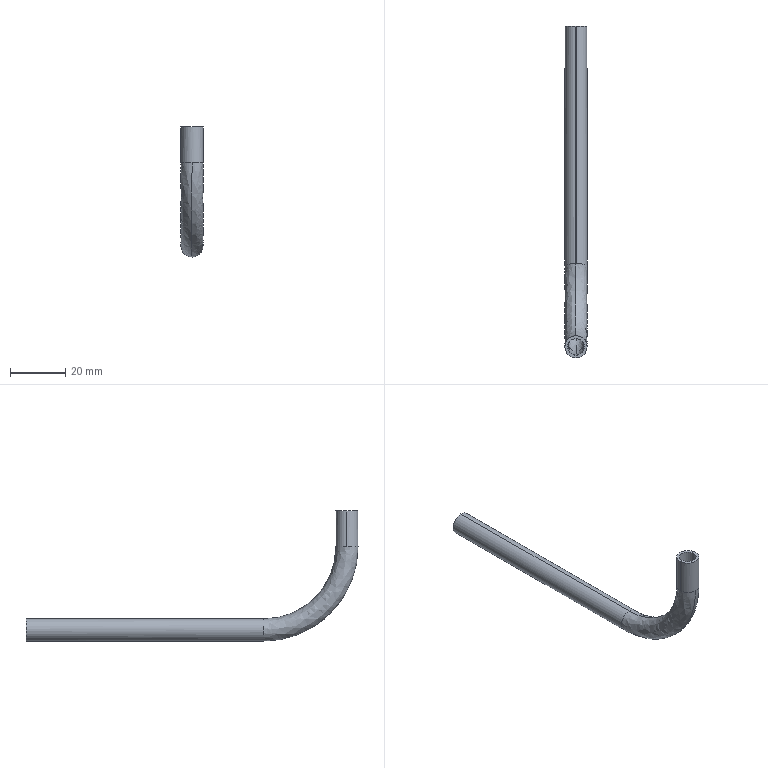Part | SolidWorks | features BaseBody 1 | 1 solid | 14 faces | box 8 x 120 x 47 mm | volume 3213 mm3 | cylinder 8 | spline 4 | plane 2 | commonest cylinder face diameters 6 x4 8 x4
STEP:
#1=CARTESIAN_POINT('',(-48.,-40.,-43.));
#2=VERTEX_POINT('',#1);
#3=CARTESIAN_POINT('',(-44.,-40.,-39.));
#4=VERTEX_POINT('',#3);
#5=CARTESIAN_POINT('',(-48.,-40.,-39.));
#6=DIRECTION('',(0.,-1.,0.));
#7=DIRECTION('',(0.,0.,-1.));
#8=AXIS2_PLACEMENT_3D('',#5,#6,#7);
#9=CIRCLE('',#8,4.);
#10=EDGE_CURVE('',#2,#4,#9,.T.);
#11=ORIENTED_EDGE('',*,*,#10,.F.);
#12=CARTESIAN_POINT('',(-48.,46.,-43.));
#13=VERTEX_POINT('',#12);
#14=CARTESIAN_POINT('',(-48.,-40.,-43.));
#15=DIRECTION('',(0.,1.,0.));
#16=VECTOR('',#15,1000.);
#17=LINE('',#14,#16);
#18=EDGE_CURVE('',#2,#13,#17,.T.);
#19=ORIENTED_EDGE('',*,*,#18,.T.);
#20=CARTESIAN_POINT('',(-48.,46.,-35.));
#21=VERTEX_POINT('',#20);
#22=CARTESIAN_POINT('',(-48.,46.,-39.));
#23=DIRECTION('',(0.,-1.,0.));
#24=DIRECTION('',(0.,0.,1.));
#25=AXIS2_PLACEMENT_3D('',#22,#23,#24);
#26=CIRCLE('',#25,4.);
#27=EDGE_CURVE('',#13,#21,#26,.T.);
#28=ORIENTED_EDGE('',*,*,#27,.T.);
#29=CARTESIAN_POINT('',(-48.,-40.,-35.));
#30=VERTEX_POINT('',#29);
#31=CARTESIAN_POINT('',(-48.,-40.,-35.));
#32=DIRECTION('',(0.,1.,0.));
#33=VECTOR('',#32,1000.);
#34=LINE('',#31,#33);
#35=EDGE_CURVE('',#30,#21,#34,.T.);
#36=ORIENTED_EDGE('',*,*,#35,.F.);
#37=CARTESIAN_POINT('',(-48.,-40.,-39.));
#38=DIRECTION('',(0.,1.,0.));
#39=DIRECTION('',(0.,0.,1.));
#40=AXIS2_PLACEMENT_3D('',#37,#38,#39);
#41=CIRCLE('',#40,4.);
#42=EDGE_CURVE('',#30,#4,#41,.T.);
#43=ORIENTED_EDGE('',*,*,#42,.T.);
#44=EDGE_LOOP('',(#11,#19,#28,#36,#43));
#45=FACE_OUTER_BOUND('',#44,.T.);
#46=CARTESIAN_POINT('',(-48.,-40.,-39.));
#47=DIRECTION('',(0.,1.,0.));
#48=DIRECTION('',(0.,0.,1.));
#49=AXIS2_PLACEMENT_3D('',#46,#47,#48);
#50=CYLINDRICAL_SURFACE('',#49,4.);
#51=ADVANCED_FACE('',(#45),#50,.T.);
#52=CARTESIAN_POINT('',(-52.,-70.,-9.));
#53=VERTEX_POINT('',#52);
#54=CARTESIAN_POINT('',(-48.001,-66.,-9.));
#55=VERTEX_POINT('',#54);
#56=CARTESIAN_POINT('',(-48.,-70.,-9.));
#57=DIRECTION('',(0.,0.,-1.));
#58=DIRECTION('',(0.,-1.,0.));
#59=AXIS2_PLACEMENT_3D('',#56,#57,#58);
#60=CIRCLE('',#59,4.);
#61=EDGE_CURVE('',#53,#55,#60,.T.);
#62=ORIENTED_EDGE('',*,*,#61,.F.);
#63=CARTESIAN_POINT('',(-52.,-70.,4.));
#64=VERTEX_POINT('',#63);
#65=CARTESIAN_POINT('',(-52.,-70.,-9.));
#66=DIRECTION('',(0.,0.,1.));
#67=VECTOR('',#66,1000.);
#68=LINE('',#65,#67);
#69=EDGE_CURVE('',#53,#64,#68,.T.);
#70=ORIENTED_EDGE('',*,*,#69,.T.);
#71=CARTESIAN_POINT('',(-44.,-70.,4.));
#72=VERTEX_POINT('',#71);
#73=CARTESIAN_POINT('',(-48.,-70.,4.));
#74=DIRECTION('',(0.,0.,-1.));
#75=DIRECTION('',(1.,0.,0.));
#76=AXIS2_PLACEMENT_3D('',#73,#74,#75);
#77=CIRCLE('',#76,4.);
#78=EDGE_CURVE('',#64,#72,#77,.T.);
#79=ORIENTED_EDGE('',*,*,#78,.T.);
#80=CARTESIAN_POINT('',(-44.,-70.,-9.));
#81=VERTEX_POINT('',#80);
#82=CARTESIAN_POINT('',(-44.,-70.,-9.));
#83=DIRECTION('',(0.,0.,1.));
#84=VECTOR('',#83,1000.);
#85=LINE('',#82,#84);
#86=EDGE_CURVE('',#81,#72,#85,.T.);
#87=ORIENTED_EDGE('',*,*,#86,.F.);
#88=CARTESIAN_POINT('',(-48.,-70.,-9.));
#89=DIRECTION('',(0.,0.,-1.));
#90=DIRECTION('',(0.,-1.,0.));
#91=AXIS2_PLACEMENT_3D('',#88,#89,#90);
#92=CIRCLE('',#91,4.);
#93=EDGE_CURVE('',#55,#81,#92,.T.);
#94=ORIENTED_EDGE('',*,*,#93,.F.);
#95=EDGE_LOOP('',(#62,#70,#79,#87,#94));
#96=FACE_OUTER_BOUND('',#95,.T.);
#97=CARTESIAN_POINT('',(-48.,-70.,-9.));
#98=DIRECTION('',(0.,0.,1.));
#99=DIRECTION('',(1.,0.,0.));
#100=AXIS2_PLACEMENT_3D('',#97,#98,#99);
#101=CYLINDRICAL_SURFACE('',#100,4.);
#102=ADVANCED_FACE('',(#96),#101,.T.);
#103=CARTESIAN_POINT('',(-48.,-40.,-42.));
#104=VERTEX_POINT('',#103);
#105=CARTESIAN_POINT('',(-48.,-40.,-36.));
#106=VERTEX_POINT('',#105);
#107=CARTESIAN_POINT('',(-48.,-40.,-39.));
#108=DIRECTION('',(0.,1.,0.));
#109=DIRECTION('',(0.,0.,1.));
#110=AXIS2_PLACEMENT_3D('',#107,#108,#109);
#111=CIRCLE('',#110,3.);
#112=EDGE_CURVE('',#104,#106,#111,.T.);
#113=ORIENTED_EDGE('',*,*,#112,.F.);
#114=CARTESIAN_POINT('',(-48.,46.,-42.));
#115=VERTEX_POINT('',#114);
#116=CARTESIAN_POINT('',(-48.,-40.,-42.));
#117=DIRECTION('',(0.,1.,0.));
#118=VECTOR('',#117,1000.);
#119=LINE('',#116,#118);
#120=EDGE_CURVE('',#104,#115,#119,.T.);
#121=ORIENTED_EDGE('',*,*,#120,.T.);
#122=CARTESIAN_POINT('',(-48.,46.,-36.));
#123=VERTEX_POINT('',#122);
#124=CARTESIAN_POINT('',(-48.,46.,-39.));
#125=DIRECTION('',(0.,-1.,0.));
#126=DIRECTION('',(0.,0.,1.));
#127=AXIS2_PLACEMENT_3D('',#124,#125,#126);
#128=CIRCLE('',#127,3.);
#129=EDGE_CURVE('',#123,#115,#128,.T.);
#130=ORIENTED_EDGE('',*,*,#129,.F.);
#131=CARTESIAN_POINT('',(-48.,-40.,-36.));
#132=DIRECTION('',(0.,1.,0.));
#133=VECTOR('',#132,1000.);
#134=LINE('',#131,#133);
#135=EDGE_CURVE('',#106,#123,#134,.T.);
#136=ORIENTED_EDGE('',*,*,#135,.F.);
#137=EDGE_LOOP('',(#113,#121,#130,#136));
#138=FACE_OUTER_BOUND('',#137,.T.);
#139=CARTESIAN_POINT('',(-48.,-40.,-39.));
#140=DIRECTION('',(0.,1.,0.));
#141=DIRECTION('',(0.,0.,1.));
#142=AXIS2_PLACEMENT_3D('',#139,#140,#141);
#143=CYLINDRICAL_SURFACE('',#142,3.);
#144=ADVANCED_FACE('',(#138),#143,.F.);
#145=CARTESIAN_POINT('',(-48.,-67.,-9.));
#146=VERTEX_POINT('',#145);
#147=CARTESIAN_POINT('',(-45.,-70.,-9.));
#148=VERTEX_POINT('',#147);
#149=CARTESIAN_POINT('',(-48.,-70.,-9.));
#150=DIRECTION('',(0.,0.,-1.));
#151=DIRECTION('',(0.,-1.,0.));
#152=AXIS2_PLACEMENT_3D('',#149,#150,#151);
#153=CIRCLE('',#152,3.);
#154=EDGE_CURVE('',#146,#148,#153,.T.);
#155=ORIENTED_EDGE('',*,*,#154,.F.);
#156=CARTESIAN_POINT('',(-48.,-40.,-9.));
#157=DIRECTION('',(1.,0.,0.));
#158=DIRECTION('',(0.,-1.,0.));
#159=AXIS2_PLACEMENT_3D('',#156,#157,#158);
#160=CIRCLE('',#159,27.);
#161=EDGE_CURVE('',#146,#106,#160,.T.);
#162=ORIENTED_EDGE('',*,*,#161,.T.);
#163=CARTESIAN_POINT('',(-48.,-40.,-39.));
#164=DIRECTION('',(0.,1.,0.));
#165=DIRECTION('',(0.,0.,1.));
#166=AXIS2_PLACEMENT_3D('',#163,#164,#165);
#167=CIRCLE('',#166,3.);
#168=EDGE_CURVE('',#106,#104,#167,.T.);
#169=ORIENTED_EDGE('',*,*,#168,.T.);
#170=CARTESIAN_POINT('',(-48.,-73.,-9.));
#171=VERTEX_POINT('',#170);
#172=CARTESIAN_POINT('',(-48.,-40.,-9.));
#173=DIRECTION('',(1.,0.,0.));
#174=DIRECTION('',(0.,-1.,0.));
#175=AXIS2_PLACEMENT_3D('',#172,#173,#174);
#176=CIRCLE('',#175,33.);
#177=EDGE_CURVE('',#171,#104,#176,.T.);
#178=ORIENTED_EDGE('',*,*,#177,.F.);
#179=CARTESIAN_POINT('',(-48.,-70.,-9.));
#180=DIRECTION('',(0.,0.,-1.));
#181=DIRECTION('',(0.,-1.,0.));
#182=AXIS2_PLACEMENT_3D('',#179,#180,#181);
#183=CIRCLE('',#182,3.);
#184=EDGE_CURVE('',#148,#171,#183,.T.);
#185=ORIENTED_EDGE('',*,*,#184,.F.);
#186=EDGE_LOOP('',(#155,#162,#169,#178,#185));
#187=FACE_OUTER_BOUND('',#186,.T.);
#188=CARTESIAN_POINT('',(-48.,-67.,-9.));
#189=CARTESIAN_POINT('',(-48.,-67.,-24.816));
#190=CARTESIAN_POINT('',(-48.,-55.816,-36.));
#191=CARTESIAN_POINT('',(-48.,-40.,-36.));
#192=CARTESIAN_POINT('',(-42.,-67.,-9.));
#193=CARTESIAN_POINT('',(-42.,-67.,-24.816));
#194=CARTESIAN_POINT('',(-42.,-55.816,-36.));
#195=CARTESIAN_POINT('',(-42.,-40.,-36.));
#196=CARTESIAN_POINT('',(-42.,-73.,-9.));
#197=CARTESIAN_POINT('',(-42.,-73.,-28.331));
#198=CARTESIAN_POINT('',(-42.,-59.331,-42.));
#199=CARTESIAN_POINT('',(-42.,-40.,-42.));
#200=CARTESIAN_POINT('',(-48.,-73.,-9.));
#201=CARTESIAN_POINT('',(-48.,-73.,-28.331));
#202=CARTESIAN_POINT('',(-48.,-59.331,-42.));
#203=CARTESIAN_POINT('',(-48.,-40.,-42.));
#204=(BOUNDED_SURFACE()B_SPLINE_SURFACE(3,3,((#188,#189,#190,#191),(#192,#193,#194,#195),(#196,#197,#198,#199),(#200,#201,#202,#203)),.UNSPECIFIED.,.F.,.F.,.T.)B_SPLINE_SURFACE_WITH_KNOTS((4,4),(4,4),(0.,1.),(0.,1.),.UNSPECIFIED.)GEOMETRIC_REPRESENTATION_ITEM()RATIONAL_B_SPLINE_SURFACE(((1.,0.8047,0.8047,1.),(0.3333,0.2682,0.2682,0.3333),(0.3333,0.2682,0.2682,0.3333),(1.,0.8047,0.8047,1.)))REPRESENTATION_ITEM('')SURFACE());
#205=ADVANCED_FACE('',(#187),#204,.F.);
#206=ORIENTED_EDGE('',*,*,#184,.T.);
#207=CARTESIAN_POINT('',(-51.,-70.,-9.));
#208=VERTEX_POINT('',#207);
#209=CARTESIAN_POINT('',(-48.,-70.,-9.));
#210=DIRECTION('',(0.,0.,-1.));
#211=DIRECTION('',(0.,-1.,0.));
#212=AXIS2_PLACEMENT_3D('',#209,#210,#211);
#213=CIRCLE('',#212,3.);
#214=EDGE_CURVE('',#171,#208,#213,.T.);
#215=ORIENTED_EDGE('',*,*,#214,.T.);
#216=CARTESIAN_POINT('',(-51.,-70.,4.));
#217=VERTEX_POINT('',#216);
#218=CARTESIAN_POINT('',(-51.,-70.,-9.));
#219=DIRECTION('',(0.,0.,1.));
#220=VECTOR('',#219,1000.);
#221=LINE('',#218,#220);
#222=EDGE_CURVE('',#208,#217,#221,.T.);
#223=ORIENTED_EDGE('',*,*,#222,.T.);
#224=CARTESIAN_POINT('',(-45.,-70.,4.));
#225=VERTEX_POINT('',#224);
#226=CARTESIAN_POINT('',(-48.,-70.,4.));
#227=DIRECTION('',(0.,0.,-1.));
#228=DIRECTION('',(1.,0.,0.));
#229=AXIS2_PLACEMENT_3D('',#226,#227,#228);
#230=CIRCLE('',#229,3.);
#231=EDGE_CURVE('',#225,#217,#230,.T.);
#232=ORIENTED_EDGE('',*,*,#231,.F.);
#233=CARTESIAN_POINT('',(-45.,-70.,-9.));
#234=DIRECTION('',(0.,0.,1.));
#235=VECTOR('',#234,1000.);
#236=LINE('',#233,#235);
#237=EDGE_CURVE('',#148,#225,#236,.T.);
#238=ORIENTED_EDGE('',*,*,#237,.F.);
#239=EDGE_LOOP('',(#206,#215,#223,#232,#238));
#240=FACE_OUTER_BOUND('',#239,.T.);
#241=CARTESIAN_POINT('',(-48.,-70.,-9.));
#242=DIRECTION('',(0.,0.,1.));
#243=DIRECTION('',(1.,0.,0.));
#244=AXIS2_PLACEMENT_3D('',#241,#242,#243);
#245=CYLINDRICAL_SURFACE('',#244,3.);
#246=ADVANCED_FACE('',(#240),#245,.F.);
#247=ORIENTED_EDGE('',*,*,#18,.F.);
#248=CARTESIAN_POINT('',(-52.,-40.,-39.));
#249=VERTEX_POINT('',#248);
#250=CARTESIAN_POINT('',(-48.,-40.,-39.));
#251=DIRECTION('',(0.,-1.,0.));
#252=DIRECTION('',(0.,0.,-1.));
#253=AXIS2_PLACEMENT_3D('',#250,#251,#252);
#254=CIRCLE('',#253,4.);
#255=EDGE_CURVE('',#249,#2,#254,.T.);
#256=ORIENTED_EDGE('',*,*,#255,.F.);
#257=CARTESIAN_POINT('',(-48.001,-40.,-35.));
#258=VERTEX_POINT('',#257);
#259=CARTESIAN_POINT('',(-48.,-40.,-39.));
#260=DIRECTION('',(0.,1.,0.));
#261=DIRECTION('',(0.,0.,1.));
#262=AXIS2_PLACEMENT_3D('',#259,#260,#261);
#263=CIRCLE('',#262,4.);
#264=EDGE_CURVE('',#249,#258,#263,.T.);
#265=ORIENTED_EDGE('',*,*,#264,.T.);
#266=CARTESIAN_POINT('',(-48.,-40.,-39.));
#267=DIRECTION('',(0.,1.,0.));
#268=DIRECTION('',(0.,0.,1.));
#269=AXIS2_PLACEMENT_3D('',#266,#267,#268);
#270=CIRCLE('',#269,4.);
#271=EDGE_CURVE('',#258,#30,#270,.T.);
#272=ORIENTED_EDGE('',*,*,#271,.T.);
#273=ORIENTED_EDGE('',*,*,#35,.T.);
#274=CARTESIAN_POINT('',(-48.,46.,-39.));
#275=DIRECTION('',(0.,-1.,0.));
#276=DIRECTION('',(0.,0.,1.));
#277=AXIS2_PLACEMENT_3D('',#274,#275,#276);
#278=CIRCLE('',#277,4.);
#279=EDGE_CURVE('',#21,#13,#278,.T.);
#280=ORIENTED_EDGE('',*,*,#279,.T.);
#281=EDGE_LOOP('',(#247,#256,#265,#272,#273,#280));
#282=FACE_OUTER_BOUND('',#281,.T.);
#283=CARTESIAN_POINT('',(-48.,-40.,-39.));
#284=DIRECTION('',(0.,1.,0.));
#285=DIRECTION('',(0.,0.,1.));
#286=AXIS2_PLACEMENT_3D('',#283,#284,#285);
#287=CYLINDRICAL_SURFACE('',#286,4.);
#288=ADVANCED_FACE('',(#282),#287,.T.);
#289=CARTESIAN_POINT('',(-48.001,-40.,-9.));
#290=DIRECTION('',(-1.,0.,0.));
#291=DIRECTION('',(0.,-1.,0.));
#292=AXIS2_PLACEMENT_3D('',#289,#290,#291);
#293=CIRCLE('',#292,26.);
#294=EDGE_CURVE('',#258,#55,#293,.T.);
#295=ORIENTED_EDGE('',*,*,#294,.T.);
#296=ORIENTED_EDGE('',*,*,#93,.T.);
#297=CARTESIAN_POINT('',(-48.,-74.,-9.));
#298=VERTEX_POINT('',#297);
#299=CARTESIAN_POINT('',(-48.,-70.,-9.));
#300=DIRECTION('',(0.,0.,-1.));
#301=DIRECTION('',(0.,-1.,0.));
#302=AXIS2_PLACEMENT_3D('',#299,#300,#301);
#303=CIRCLE('',#302,4.);
#304=EDGE_CURVE('',#81,#298,#303,.T.);
#305=ORIENTED_EDGE('',*,*,#304,.T.);
#306=CARTESIAN_POINT('',(-48.,-40.,-9.));
#307=DIRECTION('',(1.,0.,0.));
#308=DIRECTION('',(0.,-1.,0.));
#309=AXIS2_PLACEMENT_3D('',#306,#307,#308);
#310=CIRCLE('',#309,34.);
#311=EDGE_CURVE('',#298,#2,#310,.T.);
#312=ORIENTED_EDGE('',*,*,#311,.T.);
#313=ORIENTED_EDGE('',*,*,#10,.T.);
#314=ORIENTED_EDGE('',*,*,#42,.F.);
#315=ORIENTED_EDGE('',*,*,#271,.F.);
#316=EDGE_LOOP('',(#295,#296,#305,#312,#313,#314,#315));
#317=FACE_OUTER_BOUND('',#316,.T.);
#318=CARTESIAN_POINT('',(-48.001,-66.,-9.));
#319=CARTESIAN_POINT('',(-48.001,-66.,-24.23));
#320=CARTESIAN_POINT('',(-48.001,-55.23,-35.));
#321=CARTESIAN_POINT('',(-48.001,-40.,-35.));
#322=CARTESIAN_POINT('',(-45.657,-66.,-9.));
#323=CARTESIAN_POINT('',(-45.657,-66.,-24.23));
#324=CARTESIAN_POINT('',(-45.657,-55.23,-35.));
#325=CARTESIAN_POINT('',(-45.657,-40.,-35.));
#326=CARTESIAN_POINT('',(-44.,-67.656,-9.));
#327=CARTESIAN_POINT('',(-44.,-67.656,-25.201));
#328=CARTESIAN_POINT('',(-44.,-56.201,-36.656));
#329=CARTESIAN_POINT('',(-44.,-40.,-36.656));
#330=CARTESIAN_POINT('',(-44.,-70.,-9.));
#331=CARTESIAN_POINT('',(-44.,-70.,-26.573));
#332=CARTESIAN_POINT('',(-44.,-57.573,-39.));
#333=CARTESIAN_POINT('',(-44.,-40.,-39.));
#334=CARTESIAN_POINT('',(-44.,-72.343,-9.));
#335=CARTESIAN_POINT('',(-44.,-72.343,-27.946));
#336=CARTESIAN_POINT('',(-44.,-58.946,-41.343));
#337=CARTESIAN_POINT('',(-44.,-40.,-41.343));
#338=CARTESIAN_POINT('',(-45.657,-74.,-9.));
#339=CARTESIAN_POINT('',(-45.657,-74.,-28.917));
#340=CARTESIAN_POINT('',(-45.657,-59.917,-43.));
#341=CARTESIAN_POINT('',(-45.657,-40.,-43.));
#342=CARTESIAN_POINT('',(-48.,-74.,-9.));
#343=CARTESIAN_POINT('',(-48.,-74.,-28.917));
#344=CARTESIAN_POINT('',(-48.,-59.917,-43.));
#345=CARTESIAN_POINT('',(-48.,-40.,-43.));
#346=(BOUNDED_SURFACE()B_SPLINE_SURFACE(3,3,((#318,#319,#320,#321),(#322,#323,#324,#325),(#326,#327,#328,#329),(#330,#331,#332,#333),(#334,#335,#336,#337),(#338,#339,#340,#341),(#342,#343,#344,#345)),.UNSPECIFIED.,.F.,.F.,.T.)B_SPLINE_SURFACE_WITH_KNOTS((4,3,4),(4,4),(0.,0.5,1.),(0.,1.),.UNSPECIFIED.)GEOMETRIC_REPRESENTATION_ITEM()RATIONAL_B_SPLINE_SURFACE(((1.,0.8047,0.8047,1.),(0.8047,0.6476,0.6476,0.8047),(0.8047,0.6476,0.6476,0.8047),(1.,0.8047,0.8047,1.),(0.8047,0.6476,0.6476,0.8047),(0.8047,0.6476,0.6476,0.8047),(1.,0.8047,0.8047,1.)))REPRESENTATION_ITEM('')SURFACE());
#347=ADVANCED_FACE('',(#317),#346,.T.);
#348=ORIENTED_EDGE('',*,*,#311,.F.);
#349=CARTESIAN_POINT('',(-48.,-70.,-9.));
#350=DIRECTION('',(0.,0.,-1.));
#351=DIRECTION('',(0.,-1.,0.));
#352=AXIS2_PLACEMENT_3D('',#349,#350,#351);
#353=CIRCLE('',#352,4.);
#354=EDGE_CURVE('',#298,#53,#353,.T.);
#355=ORIENTED_EDGE('',*,*,#354,.T.);
#356=ORIENTED_EDGE('',*,*,#61,.T.);
#357=ORIENTED_EDGE('',*,*,#294,.F.);
#358=ORIENTED_EDGE('',*,*,#264,.F.);
#359=ORIENTED_EDGE('',*,*,#255,.T.);
#360=EDGE_LOOP('',(#348,#355,#356,#357,#358,#359));
#361=FACE_OUTER_BOUND('',#360,.T.);
#362=CARTESIAN_POINT('',(-48.,-74.,-9.));
#363=CARTESIAN_POINT('',(-48.,-74.,-28.917));
#364=CARTESIAN_POINT('',(-48.,-59.917,-43.));
#365=CARTESIAN_POINT('',(-48.,-40.,-43.));
#366=CARTESIAN_POINT('',(-55.999,-74.,-9.));
#367=CARTESIAN_POINT('',(-55.999,-74.,-28.917));
#368=CARTESIAN_POINT('',(-55.999,-59.917,-43.));
#369=CARTESIAN_POINT('',(-55.999,-40.,-43.));
#370=CARTESIAN_POINT('',(-55.999,-66.001,-9.));
#371=CARTESIAN_POINT('',(-55.999,-66.001,-24.231));
#372=CARTESIAN_POINT('',(-55.999,-55.231,-35.001));
#373=CARTESIAN_POINT('',(-55.999,-40.,-35.001));
#374=CARTESIAN_POINT('',(-48.001,-66.,-9.));
#375=CARTESIAN_POINT('',(-48.001,-66.,-24.23));
#376=CARTESIAN_POINT('',(-48.001,-55.23,-35.));
#377=CARTESIAN_POINT('',(-48.001,-40.,-35.));
#378=(BOUNDED_SURFACE()B_SPLINE_SURFACE(3,3,((#362,#363,#364,#365),(#366,#367,#368,#369),(#370,#371,#372,#373),(#374,#375,#376,#377)),.UNSPECIFIED.,.F.,.F.,.T.)B_SPLINE_SURFACE_WITH_KNOTS((4,4),(4,4),(0.,1.),(0.,1.),.UNSPECIFIED.)GEOMETRIC_REPRESENTATION_ITEM()RATIONAL_B_SPLINE_SURFACE(((1.,0.8047,0.8047,1.),(0.3334,0.2683,0.2683,0.3334),(0.3334,0.2683,0.2683,0.3334),(1.,0.8047,0.8047,1.)))REPRESENTATION_ITEM('')SURFACE());
#379=ADVANCED_FACE('',(#361),#378,.T.);
#380=ORIENTED_EDGE('',*,*,#129,.T.);
#381=CARTESIAN_POINT('',(-48.,46.,-39.));
#382=DIRECTION('',(0.,-1.,0.));
#383=DIRECTION('',(0.,0.,1.));
#384=AXIS2_PLACEMENT_3D('',#381,#382,#383);
#385=CIRCLE('',#384,3.);
#386=EDGE_CURVE('',#115,#123,#385,.T.);
#387=ORIENTED_EDGE('',*,*,#386,.T.);
#388=EDGE_LOOP('',(#380,#387));
#389=FACE_BOUND('',#388,.T.);
#390=ORIENTED_EDGE('',*,*,#279,.F.);
#391=ORIENTED_EDGE('',*,*,#27,.F.);
#392=EDGE_LOOP('',(#390,#391));
#393=FACE_OUTER_BOUND('',#392,.T.);
#394=CARTESIAN_POINT('',(-48.,46.,-39.));
#395=DIRECTION('',(0.,1.,0.));
#396=DIRECTION('',(0.,0.,1.));
#397=AXIS2_PLACEMENT_3D('',#394,#395,#396);
#398=PLANE('',#397);
#399=ADVANCED_FACE('',(#389,#393),#398,.T.);
#400=ORIENTED_EDGE('',*,*,#69,.F.);
#401=ORIENTED_EDGE('',*,*,#354,.F.);
#402=ORIENTED_EDGE('',*,*,#304,.F.);
#403=ORIENTED_EDGE('',*,*,#86,.T.);
#404=CARTESIAN_POINT('',(-48.,-70.,4.));
#405=DIRECTION('',(0.,0.,-1.));
#406=DIRECTION('',(1.,0.,0.));
#407=AXIS2_PLACEMENT_3D('',#404,#405,#406);
#408=CIRCLE('',#407,4.);
#409=EDGE_CURVE('',#72,#64,#408,.T.);
#410=ORIENTED_EDGE('',*,*,#409,.T.);
#411=EDGE_LOOP('',(#400,#401,#402,#403,#410));
#412=FACE_OUTER_BOUND('',#411,.T.);
#413=CARTESIAN_POINT('',(-48.,-70.,-9.));
#414=DIRECTION('',(0.,0.,1.));
#415=DIRECTION('',(1.,0.,0.));
#416=AXIS2_PLACEMENT_3D('',#413,#414,#415);
#417=CYLINDRICAL_SURFACE('',#416,4.);
#418=ADVANCED_FACE('',(#412),#417,.T.);
#419=ORIENTED_EDGE('',*,*,#120,.F.);
#420=ORIENTED_EDGE('',*,*,#168,.F.);
#421=ORIENTED_EDGE('',*,*,#135,.T.);
#422=ORIENTED_EDGE('',*,*,#386,.F.);
#423=EDGE_LOOP('',(#419,#420,#421,#422));
#424=FACE_OUTER_BOUND('',#423,.T.);
#425=CARTESIAN_POINT('',(-48.,-40.,-39.));
#426=DIRECTION('',(0.,1.,0.));
#427=DIRECTION('',(0.,0.,1.));
#428=AXIS2_PLACEMENT_3D('',#425,#426,#427);
#429=CYLINDRICAL_SURFACE('',#428,3.);
#430=ADVANCED_FACE('',(#424),#429,.F.);
#431=ORIENTED_EDGE('',*,*,#231,.T.);
#432=CARTESIAN_POINT('',(-48.,-70.,4.));
#433=DIRECTION('',(0.,0.,-1.));
#434=DIRECTION('',(1.,0.,0.));
#435=AXIS2_PLACEMENT_3D('',#432,#433,#434);
#436=CIRCLE('',#435,3.);
#437=EDGE_CURVE('',#217,#225,#436,.T.);
#438=ORIENTED_EDGE('',*,*,#437,.T.);
#439=EDGE_LOOP('',(#431,#438));
#440=FACE_BOUND('',#439,.T.);
#441=ORIENTED_EDGE('',*,*,#409,.F.);
#442=ORIENTED_EDGE('',*,*,#78,.F.);
#443=EDGE_LOOP('',(#441,#442));
#444=FACE_OUTER_BOUND('',#443,.T.);
#445=CARTESIAN_POINT('',(-48.,-70.,4.));
#446=DIRECTION('',(0.,0.,1.));
#447=DIRECTION('',(1.,0.,0.));
#448=AXIS2_PLACEMENT_3D('',#445,#446,#447);
#449=PLANE('',#448);
#450=ADVANCED_FACE('',(#440,#444),#449,.T.);
#451=ORIENTED_EDGE('',*,*,#161,.F.);
#452=CARTESIAN_POINT('',(-48.,-70.,-9.));
#453=DIRECTION('',(0.,0.,-1.));
#454=DIRECTION('',(0.,-1.,0.));
#455=AXIS2_PLACEMENT_3D('',#452,#453,#454);
#456=CIRCLE('',#455,3.);
#457=EDGE_CURVE('',#208,#146,#456,.T.);
#458=ORIENTED_EDGE('',*,*,#457,.F.);
#459=ORIENTED_EDGE('',*,*,#214,.F.);
#460=ORIENTED_EDGE('',*,*,#177,.T.);
#461=ORIENTED_EDGE('',*,*,#112,.T.);
#462=EDGE_LOOP('',(#451,#458,#459,#460,#461));
#463=FACE_OUTER_BOUND('',#462,.T.);
#464=CARTESIAN_POINT('',(-48.,-73.,-9.));
#465=CARTESIAN_POINT('',(-48.,-73.,-28.331));
#466=CARTESIAN_POINT('',(-48.,-59.331,-42.));
#467=CARTESIAN_POINT('',(-48.,-40.,-42.));
#468=CARTESIAN_POINT('',(-54.,-73.,-9.));
#469=CARTESIAN_POINT('',(-54.,-73.,-28.331));
#470=CARTESIAN_POINT('',(-54.,-59.331,-42.));
#471=CARTESIAN_POINT('',(-54.,-40.,-42.));
#472=CARTESIAN_POINT('',(-54.,-67.,-9.));
#473=CARTESIAN_POINT('',(-54.,-67.,-24.816));
#474=CARTESIAN_POINT('',(-54.,-55.816,-36.));
#475=CARTESIAN_POINT('',(-54.,-40.,-36.));
#476=CARTESIAN_POINT('',(-48.,-67.,-9.));
#477=CARTESIAN_POINT('',(-48.,-67.,-24.816));
#478=CARTESIAN_POINT('',(-48.,-55.816,-36.));
#479=CARTESIAN_POINT('',(-48.,-40.,-36.));
#480=(BOUNDED_SURFACE()B_SPLINE_SURFACE(3,3,((#464,#465,#466,#467),(#468,#469,#470,#471),(#472,#473,#474,#475),(#476,#477,#478,#479)),.UNSPECIFIED.,.F.,.F.,.T.)B_SPLINE_SURFACE_WITH_KNOTS((4,4),(4,4),(0.,1.),(0.,1.),.UNSPECIFIED.)GEOMETRIC_REPRESENTATION_ITEM()RATIONAL_B_SPLINE_SURFACE(((1.,0.8047,0.8047,1.),(0.3333,0.2682,0.2682,0.3333),(0.3333,0.2682,0.2682,0.3333),(1.,0.8047,0.8047,1.)))REPRESENTATION_ITEM('')SURFACE());
#481=ADVANCED_FACE('',(#463),#480,.F.);
#482=ORIENTED_EDGE('',*,*,#222,.F.);
#483=ORIENTED_EDGE('',*,*,#457,.T.);
#484=ORIENTED_EDGE('',*,*,#154,.T.);
#485=ORIENTED_EDGE('',*,*,#237,.T.);
#486=ORIENTED_EDGE('',*,*,#437,.F.);
#487=EDGE_LOOP('',(#482,#483,#484,#485,#486));
#488=FACE_OUTER_BOUND('',#487,.T.);
#489=CARTESIAN_POINT('',(-48.,-70.,-9.));
#490=DIRECTION('',(0.,0.,1.));
#491=DIRECTION('',(1.,0.,0.));
#492=AXIS2_PLACEMENT_3D('',#489,#490,#491);
#493=CYLINDRICAL_SURFACE('',#492,3.);
#494=ADVANCED_FACE('',(#488),#493,.F.);
#495=CLOSED_SHELL('',(#51,#102,#144,#205,#246,#288,#347,#379,#399,#418,#430,#450,#481,#494));
#496=MANIFOLD_SOLID_BREP('',#495);
#497=CARTESIAN_POINT('',(0.,0.,0.));
#498=DIRECTION('',(0.,0.,1.));
#499=DIRECTION('',(1.,0.,0.));
#500=AXIS2_PLACEMENT_3D('',#497,#498,#499);
#501=(LENGTH_UNIT()NAMED_UNIT(*)SI_UNIT(.MILLI.,.METRE.));
#502=UNCERTAINTY_MEASURE_WITH_UNIT(LENGTH_MEASURE(0.00001),#501,'','');
#503=(NAMED_UNIT(*)PLANE_ANGLE_UNIT()SI_UNIT($,.RADIAN.));
#504=(NAMED_UNIT(*)SI_UNIT($,.STERADIAN.)SOLID_ANGLE_UNIT());
#505=(GEOMETRIC_REPRESENTATION_CONTEXT(3)GLOBAL_UNCERTAINTY_ASSIGNED_CONTEXT((#502))GLOBAL_UNIT_ASSIGNED_CONTEXT((#501,#503,#504))REPRESENTATION_CONTEXT('',''));
#506=ADVANCED_BREP_SHAPE_REPRESENTATION('',(#496,#500),#505);